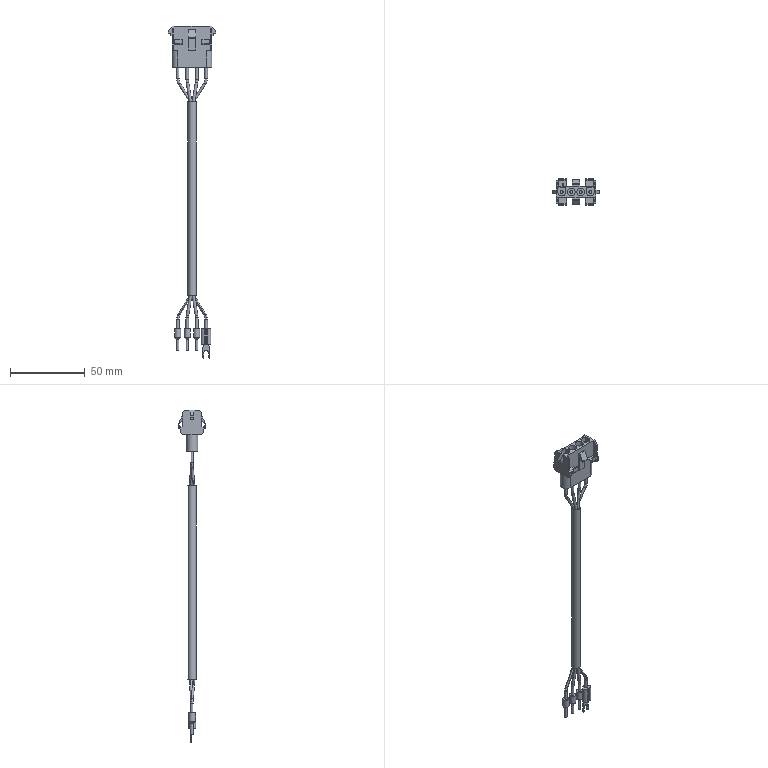Part | STEP file | BODYDZ_E-RAM6-S-640-ME30-C5 | 1 solid | 237 faces | box 31.85 x 18 x 222.5 mm | volume 8435 mm3 | plane 145 | cylinder 59 | spline 30 | cone 3 | commonest cylinder face diameters 1.8 x12 2 x8 5.25 x8 1 x7 6 x4 1.5 x3